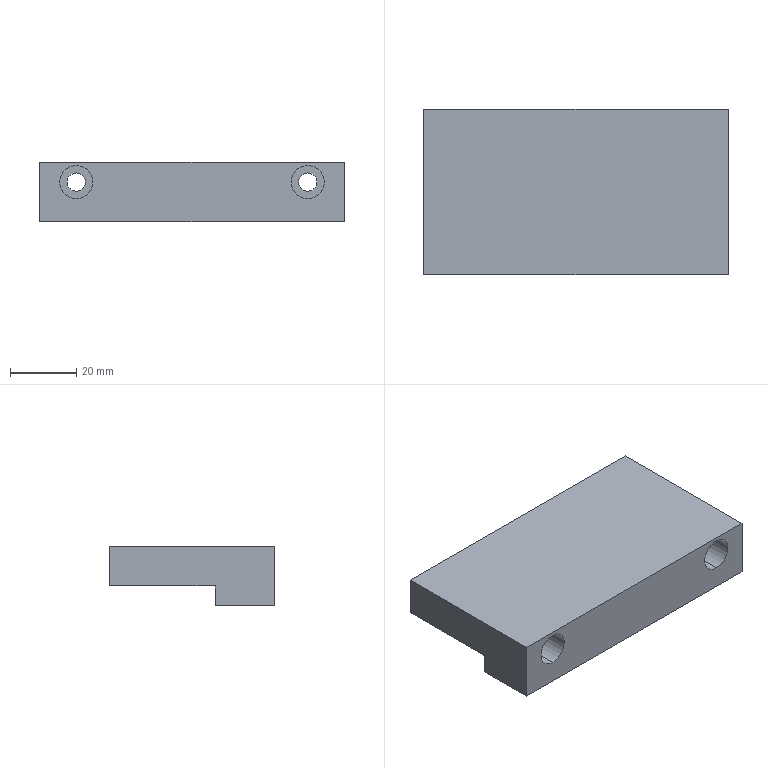Part | STEP file | 2060 Mounting plate | 1 solid | 26 faces | box 92 x 50 x 18 mm | volume 61462 mm3 | cylinder 12 | plane 10 | cone 4 | commonest cylinder face diameters 3.3 x4 5.5 x4 10 x4